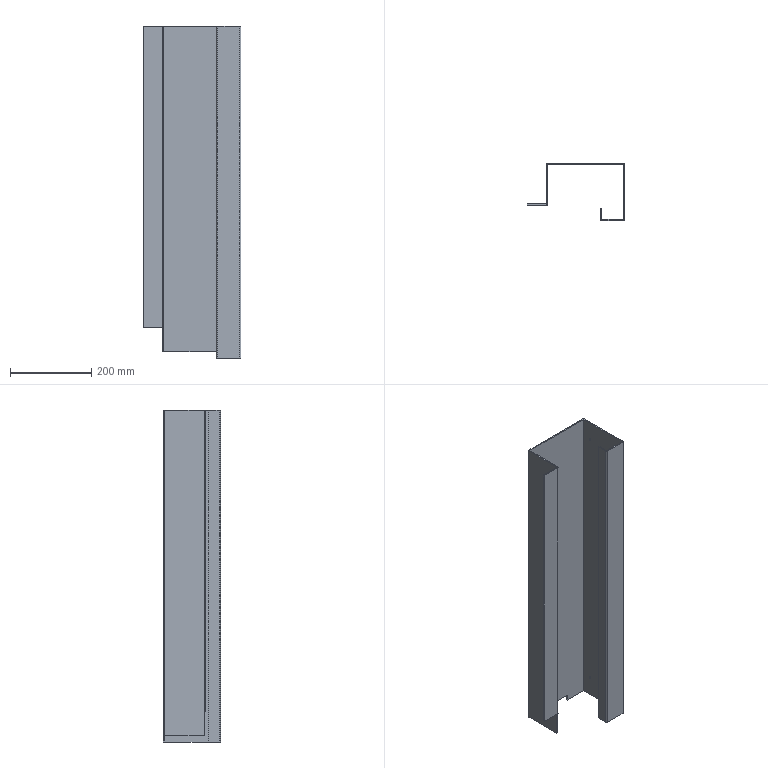Part | STEP file | TS-S40 | 1 solid | 56 faces | box 240 x 140 x 815 mm | volume 1340937 mm3 | plane 38 | cylinder 18 | commonest cylinder face diameters 5.4 x8 0.4 x5 6.4 x5